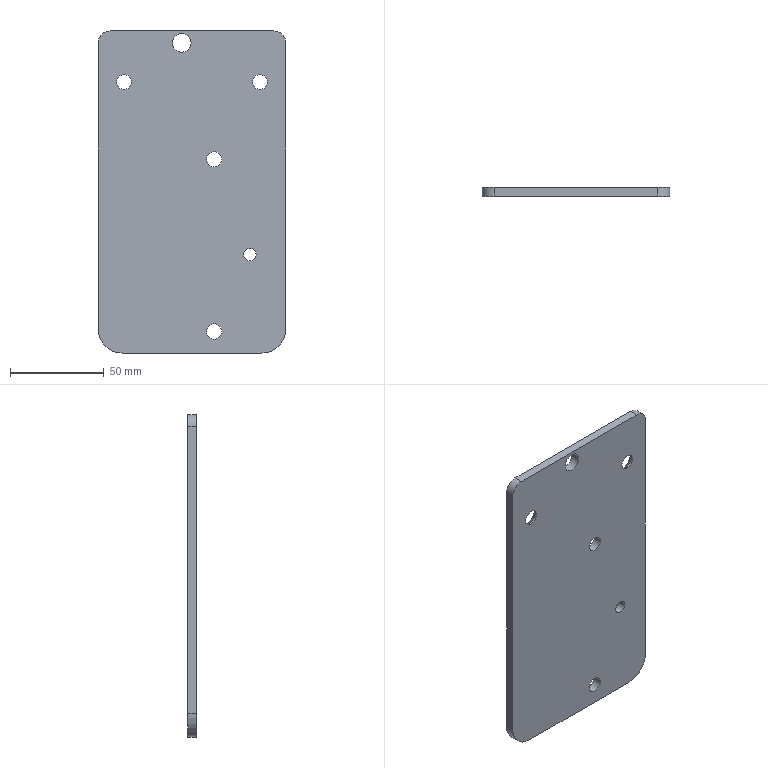Part | NX | features BREP 1 | 1 solid | 26 faces | box 99.822 x 4.763 x 171.45 mm | volume 79180 mm3 | cylinder 16 | plane 6 | cone 4 | commonest cylinder face diameters 7.938 x4 8.128 x4 6.604 x2 9.906 x2 12.7 x2 25.4 x2
STEP:
#1=CARTESIAN_POINT('',(6.35,-4.763,0.));
#2=VERTEX_POINT('',#1);
#3=CARTESIAN_POINT('',(93.472,-4.763,0.));
#4=VERTEX_POINT('',#3);
#5=CARTESIAN_POINT('',(6.35,-4.763,0.));
#6=DIRECTION('',(1.,0.,0.));
#7=VECTOR('',#6,1000.);
#8=LINE('',#5,#7);
#9=EDGE_CURVE('',#2,#4,#8,.T.);
#10=ORIENTED_EDGE('',*,*,#9,.F.);
#11=CARTESIAN_POINT('',(0.,-4.763,-6.35));
#12=VERTEX_POINT('',#11);
#13=CARTESIAN_POINT('',(6.35,-4.763,-6.35));
#14=DIRECTION('',(0.,-1.,0.));
#15=DIRECTION('',(0.,0.,1.));
#16=AXIS2_PLACEMENT_3D('',#13,#14,#15);
#17=CIRCLE('',#16,6.35);
#18=EDGE_CURVE('',#2,#12,#17,.T.);
#19=ORIENTED_EDGE('',*,*,#18,.T.);
#20=CARTESIAN_POINT('',(0.,-4.763,-158.75));
#21=VERTEX_POINT('',#20);
#22=CARTESIAN_POINT('',(0.,-4.763,-158.75));
#23=DIRECTION('',(0.,0.,1.));
#24=VECTOR('',#23,1000.);
#25=LINE('',#22,#24);
#26=EDGE_CURVE('',#21,#12,#25,.T.);
#27=ORIENTED_EDGE('',*,*,#26,.F.);
#28=CARTESIAN_POINT('',(12.7,-4.763,-171.45));
#29=VERTEX_POINT('',#28);
#30=CARTESIAN_POINT('',(12.7,-4.763,-158.75));
#31=DIRECTION('',(0.,-1.,0.));
#32=DIRECTION('',(-1.,0.,0.));
#33=AXIS2_PLACEMENT_3D('',#30,#31,#32);
#34=CIRCLE('',#33,12.7);
#35=EDGE_CURVE('',#21,#29,#34,.T.);
#36=ORIENTED_EDGE('',*,*,#35,.T.);
#37=CARTESIAN_POINT('',(87.122,-4.763,-171.45));
#38=VERTEX_POINT('',#37);
#39=CARTESIAN_POINT('',(87.122,-4.763,-171.45));
#40=DIRECTION('',(-1.,0.,0.));
#41=VECTOR('',#40,1000.);
#42=LINE('',#39,#41);
#43=EDGE_CURVE('',#38,#29,#42,.T.);
#44=ORIENTED_EDGE('',*,*,#43,.F.);
#45=CARTESIAN_POINT('',(99.822,-4.763,-158.75));
#46=VERTEX_POINT('',#45);
#47=CARTESIAN_POINT('',(87.122,-4.763,-158.75));
#48=DIRECTION('',(0.,-1.,0.));
#49=DIRECTION('',(0.,0.,-1.));
#50=AXIS2_PLACEMENT_3D('',#47,#48,#49);
#51=CIRCLE('',#50,12.7);
#52=EDGE_CURVE('',#38,#46,#51,.T.);
#53=ORIENTED_EDGE('',*,*,#52,.T.);
#54=CARTESIAN_POINT('',(99.822,-4.763,-6.35));
#55=VERTEX_POINT('',#54);
#56=CARTESIAN_POINT('',(99.822,-4.763,-6.35));
#57=DIRECTION('',(0.,0.,-1.));
#58=VECTOR('',#57,1000.);
#59=LINE('',#56,#58);
#60=EDGE_CURVE('',#55,#46,#59,.T.);
#61=ORIENTED_EDGE('',*,*,#60,.F.);
#62=CARTESIAN_POINT('',(93.472,-4.763,-6.35));
#63=DIRECTION('',(0.,-1.,0.));
#64=DIRECTION('',(1.,0.,0.));
#65=AXIS2_PLACEMENT_3D('',#62,#63,#64);
#66=CIRCLE('',#65,6.35);
#67=EDGE_CURVE('',#55,#4,#66,.T.);
#68=ORIENTED_EDGE('',*,*,#67,.T.);
#69=EDGE_LOOP('',(#10,#19,#27,#36,#44,#53,#61,#68));
#70=FACE_BOUND('',#69,.T.);
#71=CARTESIAN_POINT('',(82.137,-4.763,-27.178));
#72=VERTEX_POINT('',#71);
#73=CARTESIAN_POINT('',(90.075,-4.763,-27.178));
#74=VERTEX_POINT('',#73);
#75=CARTESIAN_POINT('',(86.106,-4.763,-27.178));
#76=DIRECTION('',(0.,-1.,0.));
#77=DIRECTION('',(-1.,0.,0.));
#78=AXIS2_PLACEMENT_3D('',#75,#76,#77);
#79=CIRCLE('',#78,3.969);
#80=EDGE_CURVE('',#72,#74,#79,.T.);
#81=ORIENTED_EDGE('',*,*,#80,.F.);
#82=CARTESIAN_POINT('',(86.106,-4.763,-27.178));
#83=DIRECTION('',(0.,-1.,0.));
#84=DIRECTION('',(1.,0.,0.));
#85=AXIS2_PLACEMENT_3D('',#82,#83,#84);
#86=CIRCLE('',#85,3.969);
#87=EDGE_CURVE('',#74,#72,#86,.T.);
#88=ORIENTED_EDGE('',*,*,#87,.F.);
#89=EDGE_LOOP('',(#81,#88));
#90=FACE_BOUND('',#89,.T.);
#91=CARTESIAN_POINT('',(57.658,-4.763,-68.326));
#92=VERTEX_POINT('',#91);
#93=CARTESIAN_POINT('',(65.786,-4.763,-68.326));
#94=VERTEX_POINT('',#93);
#95=CARTESIAN_POINT('',(61.722,-4.763,-68.326));
#96=DIRECTION('',(0.,-1.,0.));
#97=DIRECTION('',(-1.,0.,0.));
#98=AXIS2_PLACEMENT_3D('',#95,#96,#97);
#99=CIRCLE('',#98,4.064);
#100=EDGE_CURVE('',#92,#94,#99,.T.);
#101=ORIENTED_EDGE('',*,*,#100,.F.);
#102=CARTESIAN_POINT('',(61.722,-4.763,-68.326));
#103=DIRECTION('',(0.,-1.,0.));
#104=DIRECTION('',(1.,0.,0.));
#105=AXIS2_PLACEMENT_3D('',#102,#103,#104);
#106=CIRCLE('',#105,4.064);
#107=EDGE_CURVE('',#94,#92,#106,.T.);
#108=ORIENTED_EDGE('',*,*,#107,.F.);
#109=EDGE_LOOP('',(#101,#108));
#110=FACE_BOUND('',#109,.T.);
#111=CARTESIAN_POINT('',(77.47,-4.763,-119.126));
#112=VERTEX_POINT('',#111);
#113=CARTESIAN_POINT('',(84.074,-4.763,-119.126));
#114=VERTEX_POINT('',#113);
#115=CARTESIAN_POINT('',(80.772,-4.763,-119.126));
#116=DIRECTION('',(0.,-1.,0.));
#117=DIRECTION('',(-1.,0.,0.));
#118=AXIS2_PLACEMENT_3D('',#115,#116,#117);
#119=CIRCLE('',#118,3.302);
#120=EDGE_CURVE('',#112,#114,#119,.T.);
#121=ORIENTED_EDGE('',*,*,#120,.F.);
#122=CARTESIAN_POINT('',(80.772,-4.763,-119.126));
#123=DIRECTION('',(0.,-1.,0.));
#124=DIRECTION('',(1.,0.,0.));
#125=AXIS2_PLACEMENT_3D('',#122,#123,#124);
#126=CIRCLE('',#125,3.302);
#127=EDGE_CURVE('',#114,#112,#126,.T.);
#128=ORIENTED_EDGE('',*,*,#127,.F.);
#129=EDGE_LOOP('',(#121,#128));
#130=FACE_BOUND('',#129,.T.);
#131=CARTESIAN_POINT('',(57.658,-4.763,-160.02));
#132=VERTEX_POINT('',#131);
#133=CARTESIAN_POINT('',(65.786,-4.763,-160.02));
#134=VERTEX_POINT('',#133);
#135=CARTESIAN_POINT('',(61.722,-4.763,-160.02));
#136=DIRECTION('',(0.,-1.,0.));
#137=DIRECTION('',(-1.,0.,0.));
#138=AXIS2_PLACEMENT_3D('',#135,#136,#137);
#139=CIRCLE('',#138,4.064);
#140=EDGE_CURVE('',#132,#134,#139,.T.);
#141=ORIENTED_EDGE('',*,*,#140,.F.);
#142=CARTESIAN_POINT('',(61.722,-4.763,-160.02));
#143=DIRECTION('',(0.,-1.,0.));
#144=DIRECTION('',(1.,0.,0.));
#145=AXIS2_PLACEMENT_3D('',#142,#143,#144);
#146=CIRCLE('',#145,4.064);
#147=EDGE_CURVE('',#134,#132,#146,.T.);
#148=ORIENTED_EDGE('',*,*,#147,.F.);
#149=EDGE_LOOP('',(#141,#148));
#150=FACE_BOUND('',#149,.T.);
#151=CARTESIAN_POINT('',(9.747,-4.763,-27.178));
#152=VERTEX_POINT('',#151);
#153=CARTESIAN_POINT('',(17.685,-4.763,-27.178));
#154=VERTEX_POINT('',#153);
#155=CARTESIAN_POINT('',(13.716,-4.763,-27.178));
#156=DIRECTION('',(0.,-1.,0.));
#157=DIRECTION('',(-1.,0.,0.));
#158=AXIS2_PLACEMENT_3D('',#155,#156,#157);
#159=CIRCLE('',#158,3.969);
#160=EDGE_CURVE('',#152,#154,#159,.T.);
#161=ORIENTED_EDGE('',*,*,#160,.F.);
#162=CARTESIAN_POINT('',(13.716,-4.763,-27.178));
#163=DIRECTION('',(0.,-1.,0.));
#164=DIRECTION('',(1.,0.,0.));
#165=AXIS2_PLACEMENT_3D('',#162,#163,#164);
#166=CIRCLE('',#165,3.969);
#167=EDGE_CURVE('',#154,#152,#166,.T.);
#168=ORIENTED_EDGE('',*,*,#167,.F.);
#169=EDGE_LOOP('',(#161,#168));
#170=FACE_BOUND('',#169,.T.);
#171=CARTESIAN_POINT('',(39.497,-4.763,-6.35));
#172=VERTEX_POINT('',#171);
#173=CARTESIAN_POINT('',(49.403,-4.763,-6.35));
#174=VERTEX_POINT('',#173);
#175=CARTESIAN_POINT('',(44.45,-4.763,-6.35));
#176=DIRECTION('',(0.,-1.,0.));
#177=DIRECTION('',(-1.,0.,0.));
#178=AXIS2_PLACEMENT_3D('',#175,#176,#177);
#179=CIRCLE('',#178,4.953);
#180=EDGE_CURVE('',#172,#174,#179,.T.);
#181=ORIENTED_EDGE('',*,*,#180,.F.);
#182=CARTESIAN_POINT('',(44.45,-4.763,-6.35));
#183=DIRECTION('',(0.,-1.,0.));
#184=DIRECTION('',(1.,0.,0.));
#185=AXIS2_PLACEMENT_3D('',#182,#183,#184);
#186=CIRCLE('',#185,4.953);
#187=EDGE_CURVE('',#174,#172,#186,.T.);
#188=ORIENTED_EDGE('',*,*,#187,.F.);
#189=EDGE_LOOP('',(#181,#188));
#190=FACE_BOUND('',#189,.T.);
#191=CARTESIAN_POINT('',(0.,-4.763,0.));
#192=DIRECTION('',(0.,1.,0.));
#193=DIRECTION('',(1.,0.,0.));
#194=AXIS2_PLACEMENT_3D('',#191,#192,#193);
#195=PLANE('',#194);
#196=ADVANCED_FACE('',(#70,#90,#110,#130,#150,#170,#190),#195,.F.);
#197=CARTESIAN_POINT('',(17.685,-3.81,-27.178));
#198=VERTEX_POINT('',#197);
#199=CARTESIAN_POINT('',(17.685,-3.81,-27.178));
#200=DIRECTION('',(0.,-1.,0.));
#201=VECTOR('',#200,1000.);
#202=LINE('',#199,#201);
#203=EDGE_CURVE('',#154,#198,#202,.F.);
#204=ORIENTED_EDGE('',*,*,#203,.F.);
#205=ORIENTED_EDGE('',*,*,#167,.T.);
#206=CARTESIAN_POINT('',(9.747,-3.81,-27.178));
#207=VERTEX_POINT('',#206);
#208=CARTESIAN_POINT('',(9.747,-3.81,-27.178));
#209=DIRECTION('',(0.,-1.,0.));
#210=VECTOR('',#209,1000.);
#211=LINE('',#208,#210);
#212=EDGE_CURVE('',#152,#207,#211,.F.);
#213=ORIENTED_EDGE('',*,*,#212,.T.);
#214=CARTESIAN_POINT('',(13.716,-3.81,-27.178));
#215=DIRECTION('',(0.,-1.,0.));
#216=DIRECTION('',(1.,0.,0.));
#217=AXIS2_PLACEMENT_3D('',#214,#215,#216);
#218=CIRCLE('',#217,3.969);
#219=EDGE_CURVE('',#198,#207,#218,.T.);
#220=ORIENTED_EDGE('',*,*,#219,.F.);
#221=EDGE_LOOP('',(#204,#205,#213,#220));
#222=FACE_BOUND('',#221,.T.);
#223=CARTESIAN_POINT('',(13.716,0.,-27.178));
#224=DIRECTION('',(0.,-1.,0.));
#225=DIRECTION('',(1.,0.,0.));
#226=AXIS2_PLACEMENT_3D('',#223,#224,#225);
#227=CYLINDRICAL_SURFACE('',#226,3.969);
#228=ADVANCED_FACE('',(#222),#227,.F.);
#229=CARTESIAN_POINT('',(21.115,0.,-27.178));
#230=VERTEX_POINT('',#229);
#231=CARTESIAN_POINT('',(17.685,-3.81,-27.178));
#232=DIRECTION('',(0.6691,0.7431,0.));
#233=VECTOR('',#232,1000.);
#234=LINE('',#231,#233);
#235=EDGE_CURVE('',#230,#198,#234,.F.);
#236=ORIENTED_EDGE('',*,*,#235,.T.);
#237=ORIENTED_EDGE('',*,*,#219,.T.);
#238=CARTESIAN_POINT('',(6.317,0.,-27.178));
#239=VERTEX_POINT('',#238);
#240=CARTESIAN_POINT('',(9.747,-3.81,-27.178));
#241=DIRECTION('',(-0.6691,0.7431,0.));
#242=VECTOR('',#241,1000.);
#243=LINE('',#240,#242);
#244=EDGE_CURVE('',#239,#207,#243,.F.);
#245=ORIENTED_EDGE('',*,*,#244,.F.);
#246=CARTESIAN_POINT('',(13.716,0.,-27.178));
#247=DIRECTION('',(0.,1.,0.));
#248=DIRECTION('',(-1.,0.,0.));
#249=AXIS2_PLACEMENT_3D('',#246,#247,#248);
#250=CIRCLE('',#249,7.399);
#251=EDGE_CURVE('',#239,#230,#250,.T.);
#252=ORIENTED_EDGE('',*,*,#251,.T.);
#253=EDGE_LOOP('',(#236,#237,#245,#252));
#254=FACE_BOUND('',#253,.T.);
#255=CARTESIAN_POINT('',(13.716,-1.905,-27.178));
#256=DIRECTION('',(0.,1.,0.));
#257=DIRECTION('',(1.,0.,0.));
#258=AXIS2_PLACEMENT_3D('',#255,#256,#257);
#259=CONICAL_SURFACE('',#258,5.684,0.733);
#260=ADVANCED_FACE('',(#254),#259,.F.);
#261=CARTESIAN_POINT('',(99.822,0.,-6.35));
#262=VERTEX_POINT('',#261);
#263=CARTESIAN_POINT('',(99.822,0.,-158.75));
#264=VERTEX_POINT('',#263);
#265=CARTESIAN_POINT('',(99.822,0.,-6.35));
#266=DIRECTION('',(0.,0.,-1.));
#267=VECTOR('',#266,1000.);
#268=LINE('',#265,#267);
#269=EDGE_CURVE('',#262,#264,#268,.T.);
#270=ORIENTED_EDGE('',*,*,#269,.T.);
#271=CARTESIAN_POINT('',(87.122,0.,-171.45));
#272=VERTEX_POINT('',#271);
#273=CARTESIAN_POINT('',(87.122,0.,-158.75));
#274=DIRECTION('',(0.,1.,0.));
#275=DIRECTION('',(1.,0.,0.));
#276=AXIS2_PLACEMENT_3D('',#273,#274,#275);
#277=CIRCLE('',#276,12.7);
#278=EDGE_CURVE('',#264,#272,#277,.T.);
#279=ORIENTED_EDGE('',*,*,#278,.T.);
#280=CARTESIAN_POINT('',(12.7,0.,-171.45));
#281=VERTEX_POINT('',#280);
#282=CARTESIAN_POINT('',(87.122,0.,-171.45));
#283=DIRECTION('',(-1.,0.,0.));
#284=VECTOR('',#283,1000.);
#285=LINE('',#282,#284);
#286=EDGE_CURVE('',#272,#281,#285,.T.);
#287=ORIENTED_EDGE('',*,*,#286,.T.);
#288=CARTESIAN_POINT('',(0.,0.,-158.75));
#289=VERTEX_POINT('',#288);
#290=CARTESIAN_POINT('',(12.7,0.,-158.75));
#291=DIRECTION('',(0.,1.,0.));
#292=DIRECTION('',(0.,0.,-1.));
#293=AXIS2_PLACEMENT_3D('',#290,#291,#292);
#294=CIRCLE('',#293,12.7);
#295=EDGE_CURVE('',#281,#289,#294,.T.);
#296=ORIENTED_EDGE('',*,*,#295,.T.);
#297=CARTESIAN_POINT('',(0.,0.,-6.35));
#298=VERTEX_POINT('',#297);
#299=CARTESIAN_POINT('',(0.,0.,-158.75));
#300=DIRECTION('',(0.,0.,1.));
#301=VECTOR('',#300,1000.);
#302=LINE('',#299,#301);
#303=EDGE_CURVE('',#289,#298,#302,.T.);
#304=ORIENTED_EDGE('',*,*,#303,.T.);
#305=CARTESIAN_POINT('',(6.35,0.,0.));
#306=VERTEX_POINT('',#305);
#307=CARTESIAN_POINT('',(6.35,0.,-6.35));
#308=DIRECTION('',(0.,1.,0.));
#309=DIRECTION('',(-1.,0.,0.));
#310=AXIS2_PLACEMENT_3D('',#307,#308,#309);
#311=CIRCLE('',#310,6.35);
#312=EDGE_CURVE('',#298,#306,#311,.T.);
#313=ORIENTED_EDGE('',*,*,#312,.T.);
#314=CARTESIAN_POINT('',(93.472,0.,0.));
#315=VERTEX_POINT('',#314);
#316=CARTESIAN_POINT('',(6.35,0.,0.));
#317=DIRECTION('',(1.,0.,0.));
#318=VECTOR('',#317,1000.);
#319=LINE('',#316,#318);
#320=EDGE_CURVE('',#306,#315,#319,.T.);
#321=ORIENTED_EDGE('',*,*,#320,.T.);
#322=CARTESIAN_POINT('',(93.472,0.,-6.35));
#323=DIRECTION('',(0.,1.,0.));
#324=DIRECTION('',(0.,0.,1.));
#325=AXIS2_PLACEMENT_3D('',#322,#323,#324);
#326=CIRCLE('',#325,6.35);
#327=EDGE_CURVE('',#315,#262,#326,.T.);
#328=ORIENTED_EDGE('',*,*,#327,.T.);
#329=EDGE_LOOP('',(#270,#279,#287,#296,#304,#313,#321,#328));
#330=FACE_BOUND('',#329,.T.);
#331=CARTESIAN_POINT('',(77.47,0.,-119.126));
#332=VERTEX_POINT('',#331);
#333=CARTESIAN_POINT('',(84.074,0.,-119.126));
#334=VERTEX_POINT('',#333);
#335=CARTESIAN_POINT('',(80.772,0.,-119.126));
#336=DIRECTION('',(0.,-1.,0.));
#337=DIRECTION('',(-1.,0.,0.));
#338=AXIS2_PLACEMENT_3D('',#335,#336,#337);
#339=CIRCLE('',#338,3.302);
#340=EDGE_CURVE('',#332,#334,#339,.T.);
#341=ORIENTED_EDGE('',*,*,#340,.T.);
#342=CARTESIAN_POINT('',(80.772,0.,-119.126));
#343=DIRECTION('',(0.,-1.,0.));
#344=DIRECTION('',(1.,0.,0.));
#345=AXIS2_PLACEMENT_3D('',#342,#343,#344);
#346=CIRCLE('',#345,3.302);
#347=EDGE_CURVE('',#334,#332,#346,.T.);
#348=ORIENTED_EDGE('',*,*,#347,.T.);
#349=EDGE_LOOP('',(#341,#348));
#350=FACE_BOUND('',#349,.T.);
#351=CARTESIAN_POINT('',(57.658,0.,-160.02));
#352=VERTEX_POINT('',#351);
#353=CARTESIAN_POINT('',(65.786,0.,-160.02));
#354=VERTEX_POINT('',#353);
#355=CARTESIAN_POINT('',(61.722,0.,-160.02));
#356=DIRECTION('',(0.,-1.,0.));
#357=DIRECTION('',(-1.,0.,0.));
#358=AXIS2_PLACEMENT_3D('',#355,#356,#357);
#359=CIRCLE('',#358,4.064);
#360=EDGE_CURVE('',#352,#354,#359,.T.);
#361=ORIENTED_EDGE('',*,*,#360,.T.);
#362=CARTESIAN_POINT('',(61.722,0.,-160.02));
#363=DIRECTION('',(0.,-1.,0.));
#364=DIRECTION('',(1.,0.,0.));
#365=AXIS2_PLACEMENT_3D('',#362,#363,#364);
#366=CIRCLE('',#365,4.064);
#367=EDGE_CURVE('',#354,#352,#366,.T.);
#368=ORIENTED_EDGE('',*,*,#367,.T.);
#369=EDGE_LOOP('',(#361,#368));
#370=FACE_BOUND('',#369,.T.);
#371=CARTESIAN_POINT('',(57.658,0.,-68.326));
#372=VERTEX_POINT('',#371);
#373=CARTESIAN_POINT('',(65.786,0.,-68.326));
#374=VERTEX_POINT('',#373);
#375=CARTESIAN_POINT('',(61.722,0.,-68.326));
#376=DIRECTION('',(0.,-1.,0.));
#377=DIRECTION('',(-1.,0.,0.));
#378=AXIS2_PLACEMENT_3D('',#375,#376,#377);
#379=CIRCLE('',#378,4.064);
#380=EDGE_CURVE('',#372,#374,#379,.T.);
#381=ORIENTED_EDGE('',*,*,#380,.T.);
#382=CARTESIAN_POINT('',(61.722,0.,-68.326));
#383=DIRECTION('',(0.,-1.,0.));
#384=DIRECTION('',(1.,0.,0.));
#385=AXIS2_PLACEMENT_3D('',#382,#383,#384);
#386=CIRCLE('',#385,4.064);
#387=EDGE_CURVE('',#374,#372,#386,.T.);
#388=ORIENTED_EDGE('',*,*,#387,.T.);
#389=EDGE_LOOP('',(#381,#388));
#390=FACE_BOUND('',#389,.T.);
#391=CARTESIAN_POINT('',(39.497,0.,-6.35));
#392=VERTEX_POINT('',#391);
#393=CARTESIAN_POINT('',(49.403,0.,-6.35));
#394=VERTEX_POINT('',#393);
#395=CARTESIAN_POINT('',(44.45,0.,-6.35));
#396=DIRECTION('',(0.,-1.,0.));
#397=DIRECTION('',(-1.,0.,0.));
#398=AXIS2_PLACEMENT_3D('',#395,#396,#397);
#399=CIRCLE('',#398,4.953);
#400=EDGE_CURVE('',#392,#394,#399,.T.);
#401=ORIENTED_EDGE('',*,*,#400,.T.);
#402=CARTESIAN_POINT('',(44.45,0.,-6.35));
#403=DIRECTION('',(0.,-1.,0.));
#404=DIRECTION('',(1.,0.,0.));
#405=AXIS2_PLACEMENT_3D('',#402,#403,#404);
#406=CIRCLE('',#405,4.953);
#407=EDGE_CURVE('',#394,#392,#406,.T.);
#408=ORIENTED_EDGE('',*,*,#407,.T.);
#409=EDGE_LOOP('',(#401,#408));
#410=FACE_BOUND('',#409,.T.);
#411=ORIENTED_EDGE('',*,*,#251,.F.);
#412=CARTESIAN_POINT('',(13.716,0.,-27.178));
#413=DIRECTION('',(0.,1.,0.));
#414=DIRECTION('',(1.,0.,0.));
#415=AXIS2_PLACEMENT_3D('',#412,#413,#414);
#416=CIRCLE('',#415,7.399);
#417=EDGE_CURVE('',#230,#239,#416,.T.);
#418=ORIENTED_EDGE('',*,*,#417,.F.);
#419=EDGE_LOOP('',(#411,#418));
#420=FACE_BOUND('',#419,.T.);
#421=CARTESIAN_POINT('',(78.707,0.,-27.178));
#422=VERTEX_POINT('',#421);
#423=CARTESIAN_POINT('',(93.505,0.,-27.178));
#424=VERTEX_POINT('',#423);
#425=CARTESIAN_POINT('',(86.106,0.,-27.178));
#426=DIRECTION('',(0.,1.,0.));
#427=DIRECTION('',(-1.,0.,0.));
#428=AXIS2_PLACEMENT_3D('',#425,#426,#427);
#429=CIRCLE('',#428,7.399);
#430=EDGE_CURVE('',#422,#424,#429,.T.);
#431=ORIENTED_EDGE('',*,*,#430,.F.);
#432=CARTESIAN_POINT('',(86.106,0.,-27.178));
#433=DIRECTION('',(0.,1.,0.));
#434=DIRECTION('',(1.,0.,0.));
#435=AXIS2_PLACEMENT_3D('',#432,#433,#434);
#436=CIRCLE('',#435,7.399);
#437=EDGE_CURVE('',#424,#422,#436,.T.);
#438=ORIENTED_EDGE('',*,*,#437,.F.);
#439=EDGE_LOOP('',(#431,#438));
#440=FACE_BOUND('',#439,.T.);
#441=CARTESIAN_POINT('',(0.,0.,0.));
#442=DIRECTION('',(0.,1.,0.));
#443=DIRECTION('',(1.,0.,0.));
#444=AXIS2_PLACEMENT_3D('',#441,#442,#443);
#445=PLANE('',#444);
#446=ADVANCED_FACE('',(#330,#350,#370,#390,#410,#420,#440),#445,.T.);
#447=CARTESIAN_POINT('',(65.786,0.,-68.326));
#448=DIRECTION('',(0.,-1.,0.));
#449=VECTOR('',#448,1000.);
#450=LINE('',#447,#449);
#451=EDGE_CURVE('',#94,#374,#450,.F.);
#452=ORIENTED_EDGE('',*,*,#451,.F.);
#453=ORIENTED_EDGE('',*,*,#107,.T.);
#454=CARTESIAN_POINT('',(57.658,0.,-68.326));
#455=DIRECTION('',(0.,-1.,0.));
#456=VECTOR('',#455,1000.);
#457=LINE('',#454,#456);
#458=EDGE_CURVE('',#92,#372,#457,.F.);
#459=ORIENTED_EDGE('',*,*,#458,.T.);
#460=ORIENTED_EDGE('',*,*,#387,.F.);
#461=EDGE_LOOP('',(#452,#453,#459,#460));
#462=FACE_BOUND('',#461,.T.);
#463=CARTESIAN_POINT('',(61.722,0.,-68.326));
#464=DIRECTION('',(0.,-1.,0.));
#465=DIRECTION('',(1.,0.,0.));
#466=AXIS2_PLACEMENT_3D('',#463,#464,#465);
#467=CYLINDRICAL_SURFACE('',#466,4.064);
#468=ADVANCED_FACE('',(#462),#467,.F.);
#469=ORIENTED_EDGE('',*,*,#458,.F.);
#470=ORIENTED_EDGE('',*,*,#100,.T.);
#471=ORIENTED_EDGE('',*,*,#451,.T.);
#472=ORIENTED_EDGE('',*,*,#380,.F.);
#473=EDGE_LOOP('',(#469,#470,#471,#472));
#474=FACE_BOUND('',#473,.T.);
#475=CARTESIAN_POINT('',(61.722,0.,-68.326));
#476=DIRECTION('',(0.,-1.,0.));
#477=DIRECTION('',(1.,0.,0.));
#478=AXIS2_PLACEMENT_3D('',#475,#476,#477);
#479=CYLINDRICAL_SURFACE('',#478,4.064);
#480=ADVANCED_FACE('',(#474),#479,.F.);
#481=CARTESIAN_POINT('',(84.074,0.,-119.126));
#482=DIRECTION('',(0.,-1.,0.));
#483=VECTOR('',#482,1000.);
#484=LINE('',#481,#483);
#485=EDGE_CURVE('',#114,#334,#484,.F.);
#486=ORIENTED_EDGE('',*,*,#485,.F.);
#487=ORIENTED_EDGE('',*,*,#127,.T.);
#488=CARTESIAN_POINT('',(77.47,0.,-119.126));
#489=DIRECTION('',(0.,-1.,0.));
#490=VECTOR('',#489,1000.);
#491=LINE('',#488,#490);
#492=EDGE_CURVE('',#112,#332,#491,.F.);
#493=ORIENTED_EDGE('',*,*,#492,.T.);
#494=ORIENTED_EDGE('',*,*,#347,.F.);
#495=EDGE_LOOP('',(#486,#487,#493,#494));
#496=FACE_BOUND('',#495,.T.);
#497=CARTESIAN_POINT('',(80.772,0.,-119.126));
#498=DIRECTION('',(0.,-1.,0.));
#499=DIRECTION('',(1.,0.,0.));
#500=AXIS2_PLACEMENT_3D('',#497,#498,#499);
#501=CYLINDRICAL_SURFACE('',#500,3.302);
#502=ADVANCED_FACE('',(#496),#501,.F.);
#503=ORIENTED_EDGE('',*,*,#492,.F.);
#504=ORIENTED_EDGE('',*,*,#120,.T.);
#505=ORIENTED_EDGE('',*,*,#485,.T.);
#506=ORIENTED_EDGE('',*,*,#340,.F.);
#507=EDGE_LOOP('',(#503,#504,#505,#506));
#508=FACE_BOUND('',#507,.T.);
#509=CARTESIAN_POINT('',(80.772,0.,-119.126));
#510=DIRECTION('',(0.,-1.,0.));
#511=DIRECTION('',(1.,0.,0.));
#512=AXIS2_PLACEMENT_3D('',#509,#510,#511);
#513=CYLINDRICAL_SURFACE('',#512,3.302);
#514=ADVANCED_FACE('',(#508),#513,.F.);
#515=CARTESIAN_POINT('',(65.786,0.,-160.02));
#516=DIRECTION('',(0.,-1.,0.));
#517=VECTOR('',#516,1000.);
#518=LINE('',#515,#517);
#519=EDGE_CURVE('',#134,#354,#518,.F.);
#520=ORIENTED_EDGE('',*,*,#519,.F.);
#521=ORIENTED_EDGE('',*,*,#147,.T.);
#522=CARTESIAN_POINT('',(57.658,0.,-160.02));
#523=DIRECTION('',(0.,-1.,0.));
#524=VECTOR('',#523,1000.);
#525=LINE('',#522,#524);
#526=EDGE_CURVE('',#132,#352,#525,.F.);
#527=ORIENTED_EDGE('',*,*,#526,.T.);
#528=ORIENTED_EDGE('',*,*,#367,.F.);
#529=EDGE_LOOP('',(#520,#521,#527,#528));
#530=FACE_BOUND('',#529,.T.);
#531=CARTESIAN_POINT('',(61.722,0.,-160.02));
#532=DIRECTION('',(0.,-1.,0.));
#533=DIRECTION('',(1.,0.,0.));
#534=AXIS2_PLACEMENT_3D('',#531,#532,#533);
#535=CYLINDRICAL_SURFACE('',#534,4.064);
#536=ADVANCED_FACE('',(#530),#535,.F.);
#537=ORIENTED_EDGE('',*,*,#526,.F.);
#538=ORIENTED_EDGE('',*,*,#140,.T.);
#539=ORIENTED_EDGE('',*,*,#519,.T.);
#540=ORIENTED_EDGE('',*,*,#360,.F.);
#541=EDGE_LOOP('',(#537,#538,#539,#540));
#542=FACE_BOUND('',#541,.T.);
#543=CARTESIAN_POINT('',(61.722,0.,-160.02));
#544=DIRECTION('',(0.,-1.,0.));
#545=DIRECTION('',(1.,0.,0.));
#546=AXIS2_PLACEMENT_3D('',#543,#544,#545);
#547=CYLINDRICAL_SURFACE('',#546,4.064);
#548=ADVANCED_FACE('',(#542),#547,.F.);
#549=ORIENTED_EDGE('',*,*,#67,.F.);
#550=CARTESIAN_POINT('',(99.822,-4.763,-6.35));
#551=DIRECTION('',(0.,1.,0.));
#552=VECTOR('',#551,1000.);
#553=LINE('',#550,#552);
#554=EDGE_CURVE('',#55,#262,#553,.T.);
#555=ORIENTED_EDGE('',*,*,#554,.T.);
#556=ORIENTED_EDGE('',*,*,#327,.F.);
#557=CARTESIAN_POINT('',(93.472,-4.763,0.));
#558=DIRECTION('',(0.,1.,0.));
#559=VECTOR('',#558,1000.);
#560=LINE('',#557,#559);
#561=EDGE_CURVE('',#4,#315,#560,.T.);
#562=ORIENTED_EDGE('',*,*,#561,.F.);
#563=EDGE_LOOP('',(#549,#555,#556,#562));
#564=FACE_BOUND('',#563,.T.);
#565=CARTESIAN_POINT('',(93.472,-5.24,-6.35));
#566=DIRECTION('',(0.,1.,0.));
#567=DIRECTION('',(0.,0.,1.));
#568=AXIS2_PLACEMENT_3D('',#565,#566,#567);
#569=CYLINDRICAL_SURFACE('',#568,6.35);
#570=ADVANCED_FACE('',(#564),#569,.T.);
#571=ORIENTED_EDGE('',*,*,#320,.F.);
#572=CARTESIAN_POINT('',(6.35,-4.763,0.));
#573=DIRECTION('',(0.,1.,0.));
#574=VECTOR('',#573,1000.);
#575=LINE('',#572,#574);
#576=EDGE_CURVE('',#2,#306,#575,.T.);
#577=ORIENTED_EDGE('',*,*,#576,.F.);
#578=ORIENTED_EDGE('',*,*,#9,.T.);
#579=ORIENTED_EDGE('',*,*,#561,.T.);
#580=EDGE_LOOP('',(#571,#577,#578,#579));
#581=FACE_BOUND('',#580,.T.);
#582=CARTESIAN_POINT('',(49.911,-2.381,0.));
#583=DIRECTION('',(0.,0.,1.));
#584=DIRECTION('',(1.,0.,0.));
#585=AXIS2_PLACEMENT_3D('',#582,#583,#584);
#586=PLANE('',#585);
#587=ADVANCED_FACE('',(#581),#586,.T.);
#588=ORIENTED_EDGE('',*,*,#18,.F.);
#589=ORIENTED_EDGE('',*,*,#576,.T.);
#590=ORIENTED_EDGE('',*,*,#312,.F.);
#591=CARTESIAN_POINT('',(0.,-4.763,-6.35));
#592=DIRECTION('',(0.,1.,0.));
#593=VECTOR('',#592,1000.);
#594=LINE('',#591,#593);
#595=EDGE_CURVE('',#12,#298,#594,.T.);
#596=ORIENTED_EDGE('',*,*,#595,.F.);
#597=EDGE_LOOP('',(#588,#589,#590,#596));
#598=FACE_BOUND('',#597,.T.);
#599=CARTESIAN_POINT('',(6.35,-5.24,-6.35));
#600=DIRECTION('',(0.,1.,0.));
#601=DIRECTION('',(-1.,0.,0.));
#602=AXIS2_PLACEMENT_3D('',#599,#600,#601);
#603=CYLINDRICAL_SURFACE('',#602,6.35);
#604=ADVANCED_FACE('',(#598),#603,.T.);
#605=ORIENTED_EDGE('',*,*,#303,.F.);
#606=CARTESIAN_POINT('',(0.,-4.763,-158.75));
#607=DIRECTION('',(0.,1.,0.));
#608=VECTOR('',#607,1000.);
#609=LINE('',#606,#608);
#610=EDGE_CURVE('',#21,#289,#609,.T.);
#611=ORIENTED_EDGE('',*,*,#610,.F.);
#612=ORIENTED_EDGE('',*,*,#26,.T.);
#613=ORIENTED_EDGE('',*,*,#595,.T.);
#614=EDGE_LOOP('',(#605,#611,#612,#613));
#615=FACE_BOUND('',#614,.T.);
#616=CARTESIAN_POINT('',(0.,-2.381,-85.725));
#617=DIRECTION('',(-1.,0.,0.));
#618=DIRECTION('',(0.,0.,1.));
#619=AXIS2_PLACEMENT_3D('',#616,#617,#618);
#620=PLANE('',#619);
#621=ADVANCED_FACE('',(#615),#620,.T.);
#622=ORIENTED_EDGE('',*,*,#35,.F.);
#623=ORIENTED_EDGE('',*,*,#610,.T.);
#624=ORIENTED_EDGE('',*,*,#295,.F.);
#625=CARTESIAN_POINT('',(12.7,-4.763,-171.45));
#626=DIRECTION('',(0.,1.,0.));
#627=VECTOR('',#626,1000.);
#628=LINE('',#625,#627);
#629=EDGE_CURVE('',#29,#281,#628,.T.);
#630=ORIENTED_EDGE('',*,*,#629,.F.);
#631=EDGE_LOOP('',(#622,#623,#624,#630));
#632=FACE_BOUND('',#631,.T.);
#633=CARTESIAN_POINT('',(12.7,-5.028,-158.75));
#634=DIRECTION('',(0.,1.,0.));
#635=DIRECTION('',(0.,0.,-1.));
#636=AXIS2_PLACEMENT_3D('',#633,#634,#635);
#637=CYLINDRICAL_SURFACE('',#636,12.7);
#638=ADVANCED_FACE('',(#632),#637,.T.);
#639=ORIENTED_EDGE('',*,*,#43,.T.);
#640=ORIENTED_EDGE('',*,*,#629,.T.);
#641=ORIENTED_EDGE('',*,*,#286,.F.);
#642=CARTESIAN_POINT('',(87.122,-4.763,-171.45));
#643=DIRECTION('',(0.,1.,0.));
#644=VECTOR('',#643,1000.);
#645=LINE('',#642,#644);
#646=EDGE_CURVE('',#38,#272,#645,.T.);
#647=ORIENTED_EDGE('',*,*,#646,.F.);
#648=EDGE_LOOP('',(#639,#640,#641,#647));
#649=FACE_BOUND('',#648,.T.);
#650=CARTESIAN_POINT('',(49.911,-2.381,-171.45));
#651=DIRECTION('',(0.,0.,-1.));
#652=DIRECTION('',(0.,-1.,0.));
#653=AXIS2_PLACEMENT_3D('',#650,#651,#652);
#654=PLANE('',#653);
#655=ADVANCED_FACE('',(#649),#654,.T.);
#656=ORIENTED_EDGE('',*,*,#52,.F.);
#657=ORIENTED_EDGE('',*,*,#646,.T.);
#658=ORIENTED_EDGE('',*,*,#278,.F.);
#659=CARTESIAN_POINT('',(99.822,-4.763,-158.75));
#660=DIRECTION('',(0.,1.,0.));
#661=VECTOR('',#660,1000.);
#662=LINE('',#659,#661);
#663=EDGE_CURVE('',#46,#264,#662,.T.);
#664=ORIENTED_EDGE('',*,*,#663,.F.);
#665=EDGE_LOOP('',(#656,#657,#658,#664));
#666=FACE_BOUND('',#665,.T.);
#667=CARTESIAN_POINT('',(87.122,-5.028,-158.75));
#668=DIRECTION('',(0.,1.,0.));
#669=DIRECTION('',(1.,0.,0.));
#670=AXIS2_PLACEMENT_3D('',#667,#668,#669);
#671=CYLINDRICAL_SURFACE('',#670,12.7);
#672=ADVANCED_FACE('',(#666),#671,.T.);
#673=ORIENTED_EDGE('',*,*,#60,.T.);
#674=ORIENTED_EDGE('',*,*,#663,.T.);
#675=ORIENTED_EDGE('',*,*,#269,.F.);
#676=ORIENTED_EDGE('',*,*,#554,.F.);
#677=EDGE_LOOP('',(#673,#674,#675,#676));
#678=FACE_BOUND('',#677,.T.);
#679=CARTESIAN_POINT('',(99.822,-2.381,-85.725));
#680=DIRECTION('',(1.,0.,0.));
#681=DIRECTION('',(0.,1.,0.));
#682=AXIS2_PLACEMENT_3D('',#679,#680,#681);
#683=PLANE('',#682);
#684=ADVANCED_FACE('',(#678),#683,.T.);
#685=CARTESIAN_POINT('',(39.497,-4.763,-6.35));
#686=DIRECTION('',(0.,1.,0.));
#687=VECTOR('',#686,1000.);
#688=LINE('',#685,#687);
#689=EDGE_CURVE('',#172,#392,#688,.T.);
#690=ORIENTED_EDGE('',*,*,#689,.T.);
#691=ORIENTED_EDGE('',*,*,#407,.F.);
#692=CARTESIAN_POINT('',(49.403,-4.763,-6.35));
#693=DIRECTION('',(0.,1.,0.));
#694=VECTOR('',#693,1000.);
#695=LINE('',#692,#694);
#696=EDGE_CURVE('',#174,#394,#695,.T.);
#697=ORIENTED_EDGE('',*,*,#696,.F.);
#698=ORIENTED_EDGE('',*,*,#187,.T.);
#699=EDGE_LOOP('',(#690,#691,#697,#698));
#700=FACE_BOUND('',#699,.T.);
#701=CARTESIAN_POINT('',(44.45,-2.381,-6.35));
#702=DIRECTION('',(0.,-1.,0.));
#703=DIRECTION('',(1.,0.,0.));
#704=AXIS2_PLACEMENT_3D('',#701,#702,#703);
#705=CYLINDRICAL_SURFACE('',#704,4.953);
#706=ADVANCED_FACE('',(#700),#705,.F.);
#707=ORIENTED_EDGE('',*,*,#696,.T.);
#708=ORIENTED_EDGE('',*,*,#400,.F.);
#709=ORIENTED_EDGE('',*,*,#689,.F.);
#710=ORIENTED_EDGE('',*,*,#180,.T.);
#711=EDGE_LOOP('',(#707,#708,#709,#710));
#712=FACE_BOUND('',#711,.T.);
#713=CARTESIAN_POINT('',(44.45,-2.381,-6.35));
#714=DIRECTION('',(0.,-1.,0.));
#715=DIRECTION('',(-1.,0.,0.));
#716=AXIS2_PLACEMENT_3D('',#713,#714,#715);
#717=CYLINDRICAL_SURFACE('',#716,4.953);
#718=ADVANCED_FACE('',(#712),#717,.F.);
#719=ORIENTED_EDGE('',*,*,#244,.T.);
#720=CARTESIAN_POINT('',(13.716,-3.81,-27.178));
#721=DIRECTION('',(0.,-1.,0.));
#722=DIRECTION('',(-1.,0.,0.));
#723=AXIS2_PLACEMENT_3D('',#720,#721,#722);
#724=CIRCLE('',#723,3.969);
#725=EDGE_CURVE('',#207,#198,#724,.T.);
#726=ORIENTED_EDGE('',*,*,#725,.T.);
#727=ORIENTED_EDGE('',*,*,#235,.F.);
#728=ORIENTED_EDGE('',*,*,#417,.T.);
#729=EDGE_LOOP('',(#719,#726,#727,#728));
#730=FACE_BOUND('',#729,.T.);
#731=CARTESIAN_POINT('',(13.716,-1.905,-27.178));
#732=DIRECTION('',(0.,1.,0.));
#733=DIRECTION('',(1.,0.,0.));
#734=AXIS2_PLACEMENT_3D('',#731,#732,#733);
#735=CONICAL_SURFACE('',#734,5.684,0.733);
#736=ADVANCED_FACE('',(#730),#735,.F.);
#737=ORIENTED_EDGE('',*,*,#212,.F.);
#738=ORIENTED_EDGE('',*,*,#160,.T.);
#739=ORIENTED_EDGE('',*,*,#203,.T.);
#740=ORIENTED_EDGE('',*,*,#725,.F.);
#741=EDGE_LOOP('',(#737,#738,#739,#740));
#742=FACE_BOUND('',#741,.T.);
#743=CARTESIAN_POINT('',(13.716,0.,-27.178));
#744=DIRECTION('',(0.,-1.,0.));
#745=DIRECTION('',(1.,0.,0.));
#746=AXIS2_PLACEMENT_3D('',#743,#744,#745);
#747=CYLINDRICAL_SURFACE('',#746,3.969);
#748=ADVANCED_FACE('',(#742),#747,.F.);
#749=CARTESIAN_POINT('',(82.137,-3.81,-27.178));
#750=VERTEX_POINT('',#749);
#751=CARTESIAN_POINT('',(82.137,-3.81,-27.178));
#752=DIRECTION('',(-0.6691,0.7431,0.));
#753=VECTOR('',#752,1000.);
#754=LINE('',#751,#753);
#755=EDGE_CURVE('',#750,#422,#754,.T.);
#756=ORIENTED_EDGE('',*,*,#755,.F.);
#757=CARTESIAN_POINT('',(90.075,-3.81,-27.178));
#758=VERTEX_POINT('',#757);
#759=CARTESIAN_POINT('',(86.106,-3.81,-27.178));
#760=DIRECTION('',(0.,-1.,0.));
#761=DIRECTION('',(-1.,0.,0.));
#762=AXIS2_PLACEMENT_3D('',#759,#760,#761);
#763=CIRCLE('',#762,3.969);
#764=EDGE_CURVE('',#750,#758,#763,.T.);
#765=ORIENTED_EDGE('',*,*,#764,.T.);
#766=CARTESIAN_POINT('',(90.075,-3.81,-27.178));
#767=DIRECTION('',(0.6691,0.7431,0.));
#768=VECTOR('',#767,1000.);
#769=LINE('',#766,#768);
#770=EDGE_CURVE('',#758,#424,#769,.T.);
#771=ORIENTED_EDGE('',*,*,#770,.T.);
#772=ORIENTED_EDGE('',*,*,#437,.T.);
#773=EDGE_LOOP('',(#756,#765,#771,#772));
#774=FACE_BOUND('',#773,.T.);
#775=CARTESIAN_POINT('',(86.106,-1.905,-27.178));
#776=DIRECTION('',(0.,1.,0.));
#777=DIRECTION('',(1.,0.,0.));
#778=AXIS2_PLACEMENT_3D('',#775,#776,#777);
#779=CONICAL_SURFACE('',#778,5.684,0.733);
#780=ADVANCED_FACE('',(#774),#779,.F.);
#781=ORIENTED_EDGE('',*,*,#770,.F.);
#782=CARTESIAN_POINT('',(86.106,-3.81,-27.178));
#783=DIRECTION('',(0.,-1.,0.));
#784=DIRECTION('',(1.,0.,0.));
#785=AXIS2_PLACEMENT_3D('',#782,#783,#784);
#786=CIRCLE('',#785,3.969);
#787=EDGE_CURVE('',#758,#750,#786,.T.);
#788=ORIENTED_EDGE('',*,*,#787,.T.);
#789=ORIENTED_EDGE('',*,*,#755,.T.);
#790=ORIENTED_EDGE('',*,*,#430,.T.);
#791=EDGE_LOOP('',(#781,#788,#789,#790));
#792=FACE_BOUND('',#791,.T.);
#793=CARTESIAN_POINT('',(86.106,-1.905,-27.178));
#794=DIRECTION('',(0.,1.,0.));
#795=DIRECTION('',(1.,0.,0.));
#796=AXIS2_PLACEMENT_3D('',#793,#794,#795);
#797=CONICAL_SURFACE('',#796,5.684,0.733);
#798=ADVANCED_FACE('',(#792),#797,.F.);
#799=CARTESIAN_POINT('',(90.075,-3.81,-27.178));
#800=DIRECTION('',(0.,-1.,0.));
#801=VECTOR('',#800,1000.);
#802=LINE('',#799,#801);
#803=EDGE_CURVE('',#74,#758,#802,.F.);
#804=ORIENTED_EDGE('',*,*,#803,.F.);
#805=ORIENTED_EDGE('',*,*,#87,.T.);
#806=CARTESIAN_POINT('',(82.137,-3.81,-27.178));
#807=DIRECTION('',(0.,-1.,0.));
#808=VECTOR('',#807,1000.);
#809=LINE('',#806,#808);
#810=EDGE_CURVE('',#72,#750,#809,.F.);
#811=ORIENTED_EDGE('',*,*,#810,.T.);
#812=ORIENTED_EDGE('',*,*,#787,.F.);
#813=EDGE_LOOP('',(#804,#805,#811,#812));
#814=FACE_BOUND('',#813,.T.);
#815=CARTESIAN_POINT('',(86.106,0.,-27.178));
#816=DIRECTION('',(0.,-1.,0.));
#817=DIRECTION('',(1.,0.,0.));
#818=AXIS2_PLACEMENT_3D('',#815,#816,#817);
#819=CYLINDRICAL_SURFACE('',#818,3.969);
#820=ADVANCED_FACE('',(#814),#819,.F.);
#821=ORIENTED_EDGE('',*,*,#810,.F.);
#822=ORIENTED_EDGE('',*,*,#80,.T.);
#823=ORIENTED_EDGE('',*,*,#803,.T.);
#824=ORIENTED_EDGE('',*,*,#764,.F.);
#825=EDGE_LOOP('',(#821,#822,#823,#824));
#826=FACE_BOUND('',#825,.T.);
#827=CARTESIAN_POINT('',(86.106,0.,-27.178));
#828=DIRECTION('',(0.,-1.,0.));
#829=DIRECTION('',(1.,0.,0.));
#830=AXIS2_PLACEMENT_3D('',#827,#828,#829);
#831=CYLINDRICAL_SURFACE('',#830,3.969);
#832=ADVANCED_FACE('',(#826),#831,.F.);
#833=CLOSED_SHELL('',(#196,#228,#260,#446,#468,#480,#502,#514,#536,#548,#570,#587,#604,#621,#638,#655,#672,#684,#706,#718,#736,#748,#780,#798,#820,#832));
#834=MANIFOLD_SOLID_BREP('',#833);
#835=(LENGTH_UNIT()NAMED_UNIT(*)SI_UNIT(.MILLI.,.METRE.));
#836=UNCERTAINTY_MEASURE_WITH_UNIT(LENGTH_MEASURE(0.00001),#835,'','');
#837=(NAMED_UNIT(*)PLANE_ANGLE_UNIT()SI_UNIT($,.RADIAN.));
#838=(NAMED_UNIT(*)SI_UNIT($,.STERADIAN.)SOLID_ANGLE_UNIT());
#839=(GEOMETRIC_REPRESENTATION_CONTEXT(3)GLOBAL_UNCERTAINTY_ASSIGNED_CONTEXT((#836))GLOBAL_UNIT_ASSIGNED_CONTEXT((#835,#837,#838))REPRESENTATION_CONTEXT('',''));
#840=ADVANCED_BREP_SHAPE_REPRESENTATION('',(#834),#839);